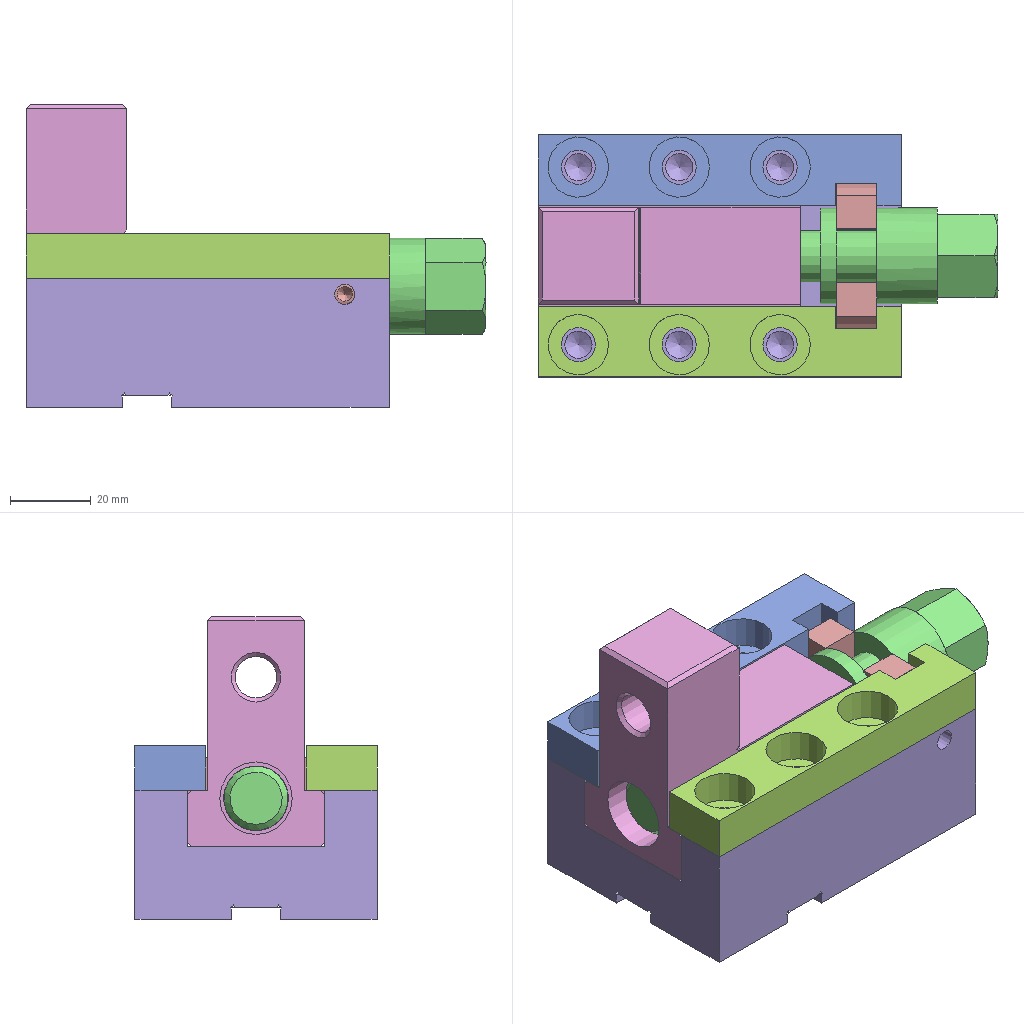Assembly | NX | 6 different items | 6 placed | box 114 x 60 x 75 mm
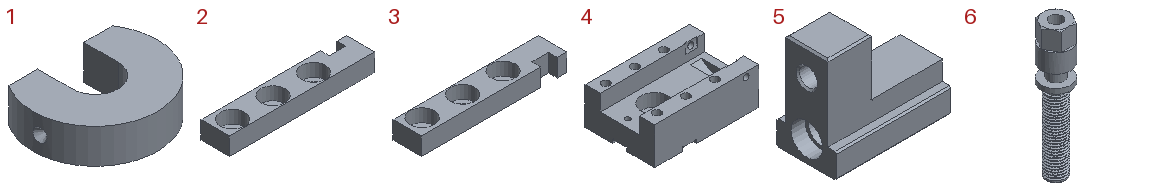Parts list (item | quantity | size | volume | features):
1 | x1 | 36.001 x 28 x 10 mm | 6442 mm3 | features DATUM_CSYS 4, CONE 2, SKETCH 2, EXTRUDE 1, MIRROR_SET 1
2 | x1 | 90 x 17.5 x 11 mm | 11956 mm3 | features EXTRACT_STRING 6, EXTRUDE 6, EXTRACT_FACE 3, DATUM_CSYS 2, Instance Feature 2, BLOCK 1, Pattern Feature 1, RECT_SLOT 1, SKETCH 1
3 | x1 | 90 x 17.5 x 11 mm | 11956 mm3 | features EXTRACT_STRING 6, EXTRUDE 6, EXTRACT_FACE 3, DATUM_CSYS 2, Instance Feature 2, BLOCK 1, Pattern Feature 1, RECT_SLOT 1, SKETCH 1
4 | x1 | 90 x 60 x 32 mm | 114243 mm3 | features DATUM_CSYS 20, SKETCH 19, HOLE PACKAGE 9, SIMPLE HOLE 9, SYMBOLIC_THREAD 9, EXTRACT_FACE 8, EXTRUDE 7, Instance Feature 6, BLOCK 2, CYLINDER 2, Pattern Feature 2, BLEND 1, CPROJ 1
5 | x1 | 65 x 34 x 57 mm | 53379 mm3 | features DATUM_CSYS 5, CHAMFER 4, SKETCH 4, BLOCK 3, CYLINDER 2, HOLE PACKAGE 2, SIMPLE HOLE 2, SYMBOLIC_THREAD 2, EXTRUDE 1
6 | x1 | 23.8 x 23.8 x 110 mm | 24209 mm3 | features CYLINDER 5, DATUM_CSYS 4, SKETCH 3, SKIN 2, CHAMFER 1, DATUM_ON_PATH 1, DATUM_PLANE 1, EXTRUDE 1, HOLE PACKAGE 1, SIMPLE HOLE 1, SYMBOLIC_THREAD 1, THREADS 1, TRIM BODY 1
Mates (type | each side: item.copy, entity, surface, feature):
Fix | 4.1 component | 2 times
Touch | 1.1 face plane Extrude(2) | 4.1 face plane Cylinder(8)
Touch | 1.1 face cylinder Extrude(2) | 4.1 face cylinder Cylinder(7)
Touch | 6.1 face plane Cylinder(5) | 1.1 face plane Extrude(2)
Touch | 3.1 edge | 4.1 face plane Block(1)
Touch | 3.1 face cylinder Extrude(4) | 4.1 face cylinder Pattern Feature [Linear] (12) / Instance[0][1]
Touch | 2.1 face plane Block(1) | 4.1 face plane Block(1)
Touch | 2.1 face cylinder Extrude(3) | 4.1 face cylinder M8 x 1.25 Threaded Hole(10)
Touch | 5.1 face plane Block(1) | 4.1 face plane Block(2) | 2 times
Touch | 5.1 face plane Block(1) | 4.1 face plane Block(1)